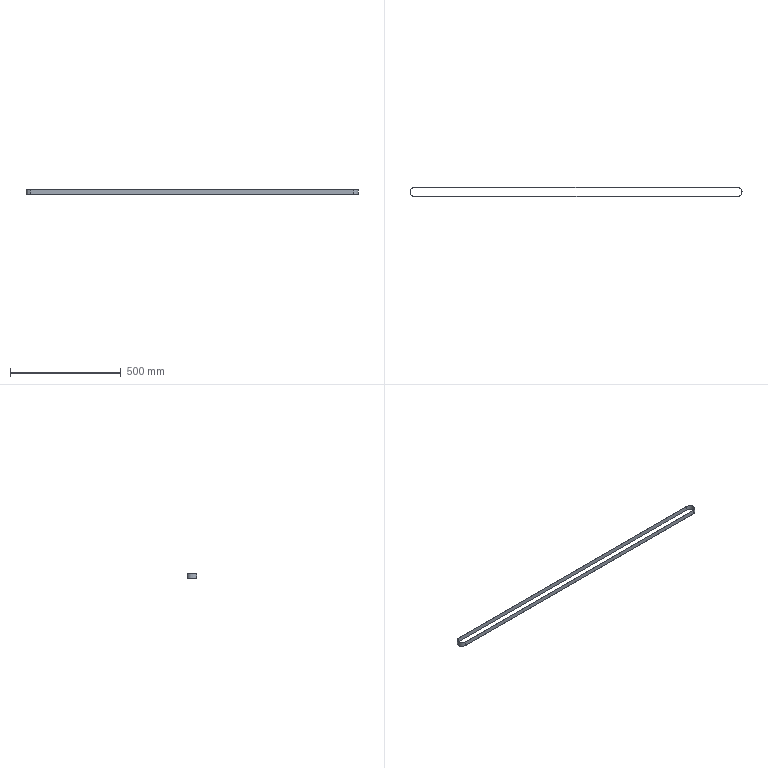Part | NX | 1 solid | 10 faces | box 1503 x 42.6 x 20 mm | volume 61014 mm3 | plane 6 | cylinder 4 | commonest cylinder face diameters 40.6 x2 42.6 x2
STEP:
#1=CARTESIAN_POINT('',(-429.48,73.3,10.));
#2=VERTEX_POINT('',#1);
#3=CARTESIAN_POINT('',(-429.48,30.7,10.));
#4=VERTEX_POINT('',#3);
#5=CARTESIAN_POINT('',(-429.48,52.,10.));
#6=DIRECTION('',(0.,0.,-1.));
#7=DIRECTION('',(-1.,0.,0.));
#8=AXIS2_PLACEMENT_3D('',#5,#6,#7);
#9=CIRCLE('',#8,21.3);
#10=EDGE_CURVE('',#2,#4,#9,.F.);
#11=ORIENTED_EDGE('',*,*,#10,.T.);
#12=CARTESIAN_POINT('',(1030.52,30.7,10.));
#13=VERTEX_POINT('',#12);
#14=CARTESIAN_POINT('',(-429.48,30.7,10.));
#15=DIRECTION('',(1.,0.,0.));
#16=VECTOR('',#15,1000.);
#17=LINE('',#14,#16);
#18=EDGE_CURVE('',#4,#13,#17,.T.);
#19=ORIENTED_EDGE('',*,*,#18,.T.);
#20=CARTESIAN_POINT('',(1030.52,73.3,10.));
#21=VERTEX_POINT('',#20);
#22=CARTESIAN_POINT('',(1030.52,52.,10.));
#23=DIRECTION('',(0.,0.,-1.));
#24=DIRECTION('',(-1.,0.,0.));
#25=AXIS2_PLACEMENT_3D('',#22,#23,#24);
#26=CIRCLE('',#25,21.3);
#27=EDGE_CURVE('',#13,#21,#26,.F.);
#28=ORIENTED_EDGE('',*,*,#27,.T.);
#29=CARTESIAN_POINT('',(-429.48,73.3,10.));
#30=DIRECTION('',(-1.,0.,0.));
#31=VECTOR('',#30,1000.);
#32=LINE('',#29,#31);
#33=EDGE_CURVE('',#21,#2,#32,.T.);
#34=ORIENTED_EDGE('',*,*,#33,.T.);
#35=EDGE_LOOP('',(#11,#19,#28,#34));
#36=FACE_BOUND('',#35,.T.);
#37=CARTESIAN_POINT('',(-429.48,72.3,10.));
#38=VERTEX_POINT('',#37);
#39=CARTESIAN_POINT('',(-429.48,31.7,10.));
#40=VERTEX_POINT('',#39);
#41=CARTESIAN_POINT('',(-429.48,52.,10.));
#42=DIRECTION('',(0.,0.,1.));
#43=DIRECTION('',(-1.,0.,0.));
#44=AXIS2_PLACEMENT_3D('',#41,#42,#43);
#45=CIRCLE('',#44,20.3);
#46=EDGE_CURVE('',#38,#40,#45,.T.);
#47=ORIENTED_EDGE('',*,*,#46,.F.);
#48=CARTESIAN_POINT('',(1030.52,72.3,10.));
#49=VERTEX_POINT('',#48);
#50=CARTESIAN_POINT('',(-429.48,72.3,10.));
#51=DIRECTION('',(-1.,0.,0.));
#52=VECTOR('',#51,1000.);
#53=LINE('',#50,#52);
#54=EDGE_CURVE('',#49,#38,#53,.T.);
#55=ORIENTED_EDGE('',*,*,#54,.F.);
#56=CARTESIAN_POINT('',(1030.52,31.7,10.));
#57=VERTEX_POINT('',#56);
#58=CARTESIAN_POINT('',(1030.52,52.,10.));
#59=DIRECTION('',(0.,0.,1.));
#60=DIRECTION('',(-1.,0.,0.));
#61=AXIS2_PLACEMENT_3D('',#58,#59,#60);
#62=CIRCLE('',#61,20.3);
#63=EDGE_CURVE('',#57,#49,#62,.T.);
#64=ORIENTED_EDGE('',*,*,#63,.F.);
#65=CARTESIAN_POINT('',(1030.52,31.7,10.));
#66=DIRECTION('',(1.,0.,0.));
#67=VECTOR('',#66,1000.);
#68=LINE('',#65,#67);
#69=EDGE_CURVE('',#40,#57,#68,.T.);
#70=ORIENTED_EDGE('',*,*,#69,.F.);
#71=EDGE_LOOP('',(#47,#55,#64,#70));
#72=FACE_BOUND('',#71,.T.);
#73=CARTESIAN_POINT('',(-429.48,52.,10.));
#74=DIRECTION('',(0.,0.,-1.));
#75=DIRECTION('',(-1.,0.,0.));
#76=AXIS2_PLACEMENT_3D('',#73,#74,#75);
#77=PLANE('',#76);
#78=ADVANCED_FACE('',(#36,#72),#77,.F.);
#79=CARTESIAN_POINT('',(-429.48,73.3,-10.));
#80=VERTEX_POINT('',#79);
#81=CARTESIAN_POINT('',(-429.48,30.7,-10.));
#82=VERTEX_POINT('',#81);
#83=CARTESIAN_POINT('',(-429.48,52.,-10.));
#84=DIRECTION('',(0.,0.,-1.));
#85=DIRECTION('',(-1.,0.,0.));
#86=AXIS2_PLACEMENT_3D('',#83,#84,#85);
#87=CIRCLE('',#86,21.3);
#88=EDGE_CURVE('',#80,#82,#87,.F.);
#89=ORIENTED_EDGE('',*,*,#88,.F.);
#90=CARTESIAN_POINT('',(1030.52,73.3,-10.));
#91=VERTEX_POINT('',#90);
#92=CARTESIAN_POINT('',(-429.48,73.3,-10.));
#93=DIRECTION('',(-1.,0.,0.));
#94=VECTOR('',#93,1000.);
#95=LINE('',#92,#94);
#96=EDGE_CURVE('',#91,#80,#95,.T.);
#97=ORIENTED_EDGE('',*,*,#96,.F.);
#98=CARTESIAN_POINT('',(1030.52,30.7,-10.));
#99=VERTEX_POINT('',#98);
#100=CARTESIAN_POINT('',(1030.52,52.,-10.));
#101=DIRECTION('',(0.,0.,-1.));
#102=DIRECTION('',(-1.,0.,0.));
#103=AXIS2_PLACEMENT_3D('',#100,#101,#102);
#104=CIRCLE('',#103,21.3);
#105=EDGE_CURVE('',#99,#91,#104,.F.);
#106=ORIENTED_EDGE('',*,*,#105,.F.);
#107=CARTESIAN_POINT('',(-429.48,30.7,-10.));
#108=DIRECTION('',(1.,0.,0.));
#109=VECTOR('',#108,1000.);
#110=LINE('',#107,#109);
#111=EDGE_CURVE('',#82,#99,#110,.T.);
#112=ORIENTED_EDGE('',*,*,#111,.F.);
#113=EDGE_LOOP('',(#89,#97,#106,#112));
#114=FACE_BOUND('',#113,.T.);
#115=CARTESIAN_POINT('',(1030.52,72.3,-10.));
#116=VERTEX_POINT('',#115);
#117=CARTESIAN_POINT('',(-429.48,72.3,-10.));
#118=VERTEX_POINT('',#117);
#119=CARTESIAN_POINT('',(-429.48,72.3,-10.));
#120=DIRECTION('',(-1.,0.,0.));
#121=VECTOR('',#120,1000.);
#122=LINE('',#119,#121);
#123=EDGE_CURVE('',#116,#118,#122,.T.);
#124=ORIENTED_EDGE('',*,*,#123,.T.);
#125=CARTESIAN_POINT('',(-429.48,31.7,-10.));
#126=VERTEX_POINT('',#125);
#127=CARTESIAN_POINT('',(-429.48,52.,-10.));
#128=DIRECTION('',(0.,0.,1.));
#129=DIRECTION('',(-1.,0.,0.));
#130=AXIS2_PLACEMENT_3D('',#127,#128,#129);
#131=CIRCLE('',#130,20.3);
#132=EDGE_CURVE('',#118,#126,#131,.T.);
#133=ORIENTED_EDGE('',*,*,#132,.T.);
#134=CARTESIAN_POINT('',(1030.52,31.7,-10.));
#135=VERTEX_POINT('',#134);
#136=CARTESIAN_POINT('',(1030.52,31.7,-10.));
#137=DIRECTION('',(1.,0.,0.));
#138=VECTOR('',#137,1000.);
#139=LINE('',#136,#138);
#140=EDGE_CURVE('',#126,#135,#139,.T.);
#141=ORIENTED_EDGE('',*,*,#140,.T.);
#142=CARTESIAN_POINT('',(1030.52,52.,-10.));
#143=DIRECTION('',(0.,0.,1.));
#144=DIRECTION('',(-1.,0.,0.));
#145=AXIS2_PLACEMENT_3D('',#142,#143,#144);
#146=CIRCLE('',#145,20.3);
#147=EDGE_CURVE('',#135,#116,#146,.T.);
#148=ORIENTED_EDGE('',*,*,#147,.T.);
#149=EDGE_LOOP('',(#124,#133,#141,#148));
#150=FACE_BOUND('',#149,.T.);
#151=CARTESIAN_POINT('',(-429.48,52.,-10.));
#152=DIRECTION('',(0.,0.,-1.));
#153=DIRECTION('',(-1.,0.,0.));
#154=AXIS2_PLACEMENT_3D('',#151,#152,#153);
#155=PLANE('',#154);
#156=ADVANCED_FACE('',(#114,#150),#155,.T.);
#157=ORIENTED_EDGE('',*,*,#88,.T.);
#158=CARTESIAN_POINT('',(-429.48,30.7,10.));
#159=DIRECTION('',(0.,0.,-1.));
#160=VECTOR('',#159,1000.);
#161=LINE('',#158,#160);
#162=EDGE_CURVE('',#4,#82,#161,.T.);
#163=ORIENTED_EDGE('',*,*,#162,.F.);
#164=ORIENTED_EDGE('',*,*,#10,.F.);
#165=CARTESIAN_POINT('',(-429.48,73.3,10.));
#166=DIRECTION('',(0.,0.,-1.));
#167=VECTOR('',#166,1000.);
#168=LINE('',#165,#167);
#169=EDGE_CURVE('',#2,#80,#168,.T.);
#170=ORIENTED_EDGE('',*,*,#169,.T.);
#171=EDGE_LOOP('',(#157,#163,#164,#170));
#172=FACE_BOUND('',#171,.T.);
#173=CARTESIAN_POINT('',(-429.48,52.,10.));
#174=DIRECTION('',(0.,0.,-1.));
#175=DIRECTION('',(-1.,0.,0.));
#176=AXIS2_PLACEMENT_3D('',#173,#174,#175);
#177=CYLINDRICAL_SURFACE('',#176,21.3);
#178=ADVANCED_FACE('',(#172),#177,.T.);
#179=ORIENTED_EDGE('',*,*,#111,.T.);
#180=CARTESIAN_POINT('',(1030.52,30.7,10.));
#181=DIRECTION('',(0.,0.,-1.));
#182=VECTOR('',#181,1000.);
#183=LINE('',#180,#182);
#184=EDGE_CURVE('',#13,#99,#183,.T.);
#185=ORIENTED_EDGE('',*,*,#184,.F.);
#186=ORIENTED_EDGE('',*,*,#18,.F.);
#187=ORIENTED_EDGE('',*,*,#162,.T.);
#188=EDGE_LOOP('',(#179,#185,#186,#187));
#189=FACE_BOUND('',#188,.T.);
#190=CARTESIAN_POINT('',(-429.48,30.7,10.));
#191=DIRECTION('',(0.,1.,0.));
#192=DIRECTION('',(0.,0.,1.));
#193=AXIS2_PLACEMENT_3D('',#190,#191,#192);
#194=PLANE('',#193);
#195=ADVANCED_FACE('',(#189),#194,.F.);
#196=ORIENTED_EDGE('',*,*,#105,.T.);
#197=CARTESIAN_POINT('',(1030.52,73.3,10.));
#198=DIRECTION('',(0.,0.,-1.));
#199=VECTOR('',#198,1000.);
#200=LINE('',#197,#199);
#201=EDGE_CURVE('',#21,#91,#200,.T.);
#202=ORIENTED_EDGE('',*,*,#201,.F.);
#203=ORIENTED_EDGE('',*,*,#27,.F.);
#204=ORIENTED_EDGE('',*,*,#184,.T.);
#205=EDGE_LOOP('',(#196,#202,#203,#204));
#206=FACE_BOUND('',#205,.T.);
#207=CARTESIAN_POINT('',(1030.52,52.,10.));
#208=DIRECTION('',(0.,0.,-1.));
#209=DIRECTION('',(-1.,0.,0.));
#210=AXIS2_PLACEMENT_3D('',#207,#208,#209);
#211=CYLINDRICAL_SURFACE('',#210,21.3);
#212=ADVANCED_FACE('',(#206),#211,.T.);
#213=ORIENTED_EDGE('',*,*,#96,.T.);
#214=ORIENTED_EDGE('',*,*,#169,.F.);
#215=ORIENTED_EDGE('',*,*,#33,.F.);
#216=ORIENTED_EDGE('',*,*,#201,.T.);
#217=EDGE_LOOP('',(#213,#214,#215,#216));
#218=FACE_BOUND('',#217,.T.);
#219=CARTESIAN_POINT('',(-429.48,73.3,10.));
#220=DIRECTION('',(0.,-1.,0.));
#221=DIRECTION('',(0.,0.,-1.));
#222=AXIS2_PLACEMENT_3D('',#219,#220,#221);
#223=PLANE('',#222);
#224=ADVANCED_FACE('',(#218),#223,.F.);
#225=ORIENTED_EDGE('',*,*,#132,.F.);
#226=CARTESIAN_POINT('',(-429.48,72.3,10.));
#227=DIRECTION('',(0.,0.,-1.));
#228=VECTOR('',#227,1000.);
#229=LINE('',#226,#228);
#230=EDGE_CURVE('',#38,#118,#229,.T.);
#231=ORIENTED_EDGE('',*,*,#230,.F.);
#232=ORIENTED_EDGE('',*,*,#46,.T.);
#233=CARTESIAN_POINT('',(-429.48,31.7,10.));
#234=DIRECTION('',(0.,0.,-1.));
#235=VECTOR('',#234,1000.);
#236=LINE('',#233,#235);
#237=EDGE_CURVE('',#40,#126,#236,.T.);
#238=ORIENTED_EDGE('',*,*,#237,.T.);
#239=EDGE_LOOP('',(#225,#231,#232,#238));
#240=FACE_BOUND('',#239,.T.);
#241=CARTESIAN_POINT('',(-429.48,52.,10.));
#242=DIRECTION('',(0.,0.,-1.));
#243=DIRECTION('',(-1.,0.,0.));
#244=AXIS2_PLACEMENT_3D('',#241,#242,#243);
#245=CYLINDRICAL_SURFACE('',#244,20.3);
#246=ADVANCED_FACE('',(#240),#245,.F.);
#247=ORIENTED_EDGE('',*,*,#140,.F.);
#248=ORIENTED_EDGE('',*,*,#237,.F.);
#249=ORIENTED_EDGE('',*,*,#69,.T.);
#250=CARTESIAN_POINT('',(1030.52,31.7,10.));
#251=DIRECTION('',(0.,0.,-1.));
#252=VECTOR('',#251,1000.);
#253=LINE('',#250,#252);
#254=EDGE_CURVE('',#57,#135,#253,.T.);
#255=ORIENTED_EDGE('',*,*,#254,.T.);
#256=EDGE_LOOP('',(#247,#248,#249,#255));
#257=FACE_BOUND('',#256,.T.);
#258=CARTESIAN_POINT('',(1030.52,31.7,10.));
#259=DIRECTION('',(0.,1.,0.));
#260=DIRECTION('',(0.,0.,1.));
#261=AXIS2_PLACEMENT_3D('',#258,#259,#260);
#262=PLANE('',#261);
#263=ADVANCED_FACE('',(#257),#262,.T.);
#264=ORIENTED_EDGE('',*,*,#147,.F.);
#265=ORIENTED_EDGE('',*,*,#254,.F.);
#266=ORIENTED_EDGE('',*,*,#63,.T.);
#267=CARTESIAN_POINT('',(1030.52,72.3,10.));
#268=DIRECTION('',(0.,0.,-1.));
#269=VECTOR('',#268,1000.);
#270=LINE('',#267,#269);
#271=EDGE_CURVE('',#49,#116,#270,.T.);
#272=ORIENTED_EDGE('',*,*,#271,.T.);
#273=EDGE_LOOP('',(#264,#265,#266,#272));
#274=FACE_BOUND('',#273,.T.);
#275=CARTESIAN_POINT('',(1030.52,52.,10.));
#276=DIRECTION('',(0.,0.,-1.));
#277=DIRECTION('',(-1.,0.,0.));
#278=AXIS2_PLACEMENT_3D('',#275,#276,#277);
#279=CYLINDRICAL_SURFACE('',#278,20.3);
#280=ADVANCED_FACE('',(#274),#279,.F.);
#281=ORIENTED_EDGE('',*,*,#123,.F.);
#282=ORIENTED_EDGE('',*,*,#271,.F.);
#283=ORIENTED_EDGE('',*,*,#54,.T.);
#284=ORIENTED_EDGE('',*,*,#230,.T.);
#285=EDGE_LOOP('',(#281,#282,#283,#284));
#286=FACE_BOUND('',#285,.T.);
#287=CARTESIAN_POINT('',(-429.48,72.3,10.));
#288=DIRECTION('',(0.,-1.,0.));
#289=DIRECTION('',(0.,0.,-1.));
#290=AXIS2_PLACEMENT_3D('',#287,#288,#289);
#291=PLANE('',#290);
#292=ADVANCED_FACE('',(#286),#291,.T.);
#293=CLOSED_SHELL('',(#78,#156,#178,#195,#212,#224,#246,#263,#280,#292));
#294=MANIFOLD_SOLID_BREP('',#293);
#295=(LENGTH_UNIT()NAMED_UNIT(*)SI_UNIT(.MILLI.,.METRE.));
#296=UNCERTAINTY_MEASURE_WITH_UNIT(LENGTH_MEASURE(0.00001),#295,'','');
#297=(NAMED_UNIT(*)PLANE_ANGLE_UNIT()SI_UNIT($,.RADIAN.));
#298=(NAMED_UNIT(*)SI_UNIT($,.STERADIAN.)SOLID_ANGLE_UNIT());
#299=(GEOMETRIC_REPRESENTATION_CONTEXT(3)GLOBAL_UNCERTAINTY_ASSIGNED_CONTEXT((#296))GLOBAL_UNIT_ASSIGNED_CONTEXT((#295,#297,#298))REPRESENTATION_CONTEXT('',''));
#300=ADVANCED_BREP_SHAPE_REPRESENTATION('',(#294),#299);